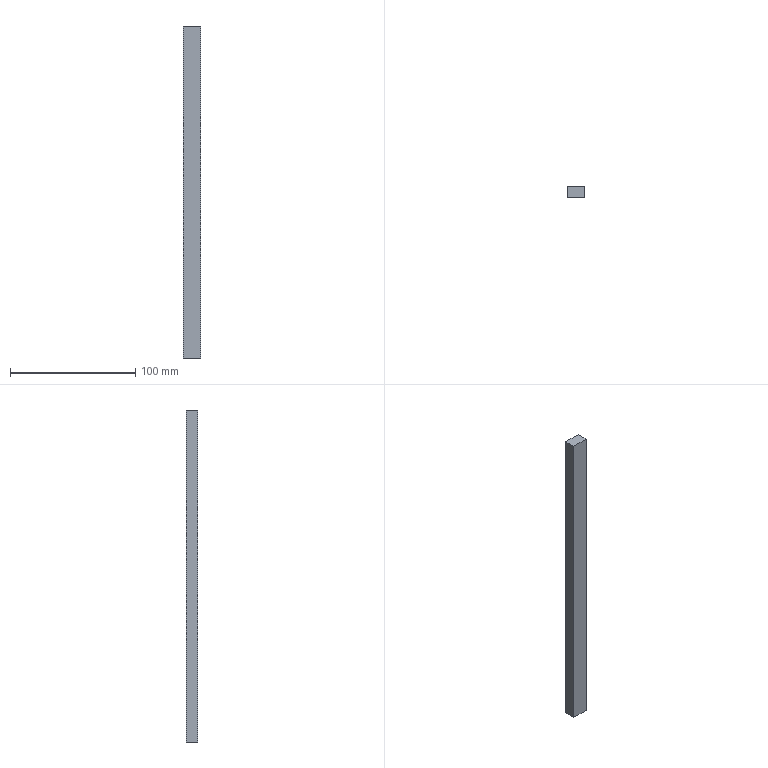Part | SolidWorks | features Extrusion 1 | 1 solid | 6 faces | box 14 x 9 x 265 mm | volume 33390 mm3 | plane 6
STEP:
#1=CARTESIAN_POINT('',(514.231,164.944,-925.693));
#2=VERTEX_POINT('',#1);
#3=CARTESIAN_POINT('',(514.231,164.944,-660.693));
#4=VERTEX_POINT('',#3);
#5=CARTESIAN_POINT('',(514.231,164.944,-925.693));
#6=DIRECTION('',(0.,0.,1.));
#7=VECTOR('',#6,1000.);
#8=LINE('',#5,#7);
#9=EDGE_CURVE('',#2,#4,#8,.T.);
#10=ORIENTED_EDGE('',*,*,#9,.F.);
#11=CARTESIAN_POINT('',(514.231,155.944,-925.693));
#12=VERTEX_POINT('',#11);
#13=CARTESIAN_POINT('',(514.231,155.944,-925.693));
#14=DIRECTION('',(0.,1.,0.));
#15=VECTOR('',#14,1000.);
#16=LINE('',#13,#15);
#17=EDGE_CURVE('',#12,#2,#16,.T.);
#18=ORIENTED_EDGE('',*,*,#17,.F.);
#19=CARTESIAN_POINT('',(514.231,155.944,-660.693));
#20=VERTEX_POINT('',#19);
#21=CARTESIAN_POINT('',(514.231,155.944,-925.693));
#22=DIRECTION('',(0.,0.,1.));
#23=VECTOR('',#22,1000.);
#24=LINE('',#21,#23);
#25=EDGE_CURVE('',#12,#20,#24,.T.);
#26=ORIENTED_EDGE('',*,*,#25,.T.);
#27=CARTESIAN_POINT('',(514.231,155.944,-660.693));
#28=DIRECTION('',(0.,1.,0.));
#29=VECTOR('',#28,1000.);
#30=LINE('',#27,#29);
#31=EDGE_CURVE('',#20,#4,#30,.T.);
#32=ORIENTED_EDGE('',*,*,#31,.T.);
#33=EDGE_LOOP('',(#10,#18,#26,#32));
#34=FACE_OUTER_BOUND('',#33,.T.);
#35=CARTESIAN_POINT('',(514.231,155.944,-925.693));
#36=DIRECTION('',(-1.,0.,0.));
#37=DIRECTION('',(0.,0.,1.));
#38=AXIS2_PLACEMENT_3D('',#35,#36,#37);
#39=PLANE('',#38);
#40=ADVANCED_FACE('',(#34),#39,.T.);
#41=CARTESIAN_POINT('',(528.231,164.944,-925.693));
#42=VERTEX_POINT('',#41);
#43=CARTESIAN_POINT('',(528.231,164.944,-925.693));
#44=DIRECTION('',(-1.,0.,0.));
#45=VECTOR('',#44,1000.);
#46=LINE('',#43,#45);
#47=EDGE_CURVE('',#42,#2,#46,.T.);
#48=ORIENTED_EDGE('',*,*,#47,.F.);
#49=CARTESIAN_POINT('',(528.231,155.944,-925.693));
#50=VERTEX_POINT('',#49);
#51=CARTESIAN_POINT('',(528.231,155.944,-925.693));
#52=DIRECTION('',(0.,1.,0.));
#53=VECTOR('',#52,1000.);
#54=LINE('',#51,#53);
#55=EDGE_CURVE('',#50,#42,#54,.T.);
#56=ORIENTED_EDGE('',*,*,#55,.F.);
#57=CARTESIAN_POINT('',(528.231,155.944,-925.693));
#58=DIRECTION('',(-1.,0.,0.));
#59=VECTOR('',#58,1000.);
#60=LINE('',#57,#59);
#61=EDGE_CURVE('',#50,#12,#60,.T.);
#62=ORIENTED_EDGE('',*,*,#61,.T.);
#63=ORIENTED_EDGE('',*,*,#17,.T.);
#64=EDGE_LOOP('',(#48,#56,#62,#63));
#65=FACE_OUTER_BOUND('',#64,.T.);
#66=CARTESIAN_POINT('',(528.231,155.944,-925.693));
#67=DIRECTION('',(0.,0.,-1.));
#68=DIRECTION('',(-1.,0.,0.));
#69=AXIS2_PLACEMENT_3D('',#66,#67,#68);
#70=PLANE('',#69);
#71=ADVANCED_FACE('',(#65),#70,.T.);
#72=CARTESIAN_POINT('',(528.231,164.944,-660.693));
#73=VERTEX_POINT('',#72);
#74=CARTESIAN_POINT('',(528.231,164.944,-660.693));
#75=DIRECTION('',(0.,0.,-1.));
#76=VECTOR('',#75,1000.);
#77=LINE('',#74,#76);
#78=EDGE_CURVE('',#73,#42,#77,.T.);
#79=ORIENTED_EDGE('',*,*,#78,.F.);
#80=CARTESIAN_POINT('',(528.231,155.944,-660.693));
#81=VERTEX_POINT('',#80);
#82=CARTESIAN_POINT('',(528.231,155.944,-660.693));
#83=DIRECTION('',(0.,1.,0.));
#84=VECTOR('',#83,1000.);
#85=LINE('',#82,#84);
#86=EDGE_CURVE('',#81,#73,#85,.T.);
#87=ORIENTED_EDGE('',*,*,#86,.F.);
#88=CARTESIAN_POINT('',(528.231,155.944,-660.693));
#89=DIRECTION('',(0.,0.,-1.));
#90=VECTOR('',#89,1000.);
#91=LINE('',#88,#90);
#92=EDGE_CURVE('',#81,#50,#91,.T.);
#93=ORIENTED_EDGE('',*,*,#92,.T.);
#94=ORIENTED_EDGE('',*,*,#55,.T.);
#95=EDGE_LOOP('',(#79,#87,#93,#94));
#96=FACE_OUTER_BOUND('',#95,.T.);
#97=CARTESIAN_POINT('',(528.231,155.944,-660.693));
#98=DIRECTION('',(1.,0.,0.));
#99=DIRECTION('',(0.,0.,-1.));
#100=AXIS2_PLACEMENT_3D('',#97,#98,#99);
#101=PLANE('',#100);
#102=ADVANCED_FACE('',(#96),#101,.T.);
#103=CARTESIAN_POINT('',(514.231,164.944,-660.693));
#104=DIRECTION('',(1.,0.,0.));
#105=VECTOR('',#104,1000.);
#106=LINE('',#103,#105);
#107=EDGE_CURVE('',#4,#73,#106,.T.);
#108=ORIENTED_EDGE('',*,*,#107,.F.);
#109=ORIENTED_EDGE('',*,*,#31,.F.);
#110=CARTESIAN_POINT('',(514.231,155.944,-660.693));
#111=DIRECTION('',(1.,0.,0.));
#112=VECTOR('',#111,1000.);
#113=LINE('',#110,#112);
#114=EDGE_CURVE('',#20,#81,#113,.T.);
#115=ORIENTED_EDGE('',*,*,#114,.T.);
#116=ORIENTED_EDGE('',*,*,#86,.T.);
#117=EDGE_LOOP('',(#108,#109,#115,#116));
#118=FACE_OUTER_BOUND('',#117,.T.);
#119=CARTESIAN_POINT('',(514.231,155.944,-660.693));
#120=DIRECTION('',(0.,0.,1.));
#121=DIRECTION('',(1.,0.,0.));
#122=AXIS2_PLACEMENT_3D('',#119,#120,#121);
#123=PLANE('',#122);
#124=ADVANCED_FACE('',(#118),#123,.T.);
#125=ORIENTED_EDGE('',*,*,#25,.F.);
#126=ORIENTED_EDGE('',*,*,#61,.F.);
#127=ORIENTED_EDGE('',*,*,#92,.F.);
#128=ORIENTED_EDGE('',*,*,#114,.F.);
#129=EDGE_LOOP('',(#125,#126,#127,#128));
#130=FACE_OUTER_BOUND('',#129,.T.);
#131=CARTESIAN_POINT('',(0.,155.944,0.));
#132=DIRECTION('',(0.,1.,0.));
#133=DIRECTION('',(0.,0.,1.));
#134=AXIS2_PLACEMENT_3D('',#131,#132,#133);
#135=PLANE('',#134);
#136=ADVANCED_FACE('',(#130),#135,.F.);
#137=ORIENTED_EDGE('',*,*,#9,.T.);
#138=ORIENTED_EDGE('',*,*,#107,.T.);
#139=ORIENTED_EDGE('',*,*,#78,.T.);
#140=ORIENTED_EDGE('',*,*,#47,.T.);
#141=EDGE_LOOP('',(#137,#138,#139,#140));
#142=FACE_OUTER_BOUND('',#141,.T.);
#143=CARTESIAN_POINT('',(0.,164.944,0.));
#144=DIRECTION('',(0.,1.,0.));
#145=DIRECTION('',(0.,0.,1.));
#146=AXIS2_PLACEMENT_3D('',#143,#144,#145);
#147=PLANE('',#146);
#148=ADVANCED_FACE('',(#142),#147,.T.);
#149=CLOSED_SHELL('',(#40,#71,#102,#124,#136,#148));
#150=MANIFOLD_SOLID_BREP('',#149);
#151=CARTESIAN_POINT('',(0.,0.,0.));
#152=DIRECTION('',(0.,0.,1.));
#153=DIRECTION('',(1.,0.,0.));
#154=AXIS2_PLACEMENT_3D('',#151,#152,#153);
#155=(LENGTH_UNIT()NAMED_UNIT(*)SI_UNIT(.MILLI.,.METRE.));
#156=UNCERTAINTY_MEASURE_WITH_UNIT(LENGTH_MEASURE(0.00001),#155,'','');
#157=(NAMED_UNIT(*)PLANE_ANGLE_UNIT()SI_UNIT($,.RADIAN.));
#158=(NAMED_UNIT(*)SI_UNIT($,.STERADIAN.)SOLID_ANGLE_UNIT());
#159=(GEOMETRIC_REPRESENTATION_CONTEXT(3)GLOBAL_UNCERTAINTY_ASSIGNED_CONTEXT((#156))GLOBAL_UNIT_ASSIGNED_CONTEXT((#155,#157,#158))REPRESENTATION_CONTEXT('',''));
#160=ADVANCED_BREP_SHAPE_REPRESENTATION('',(#150,#154),#159);